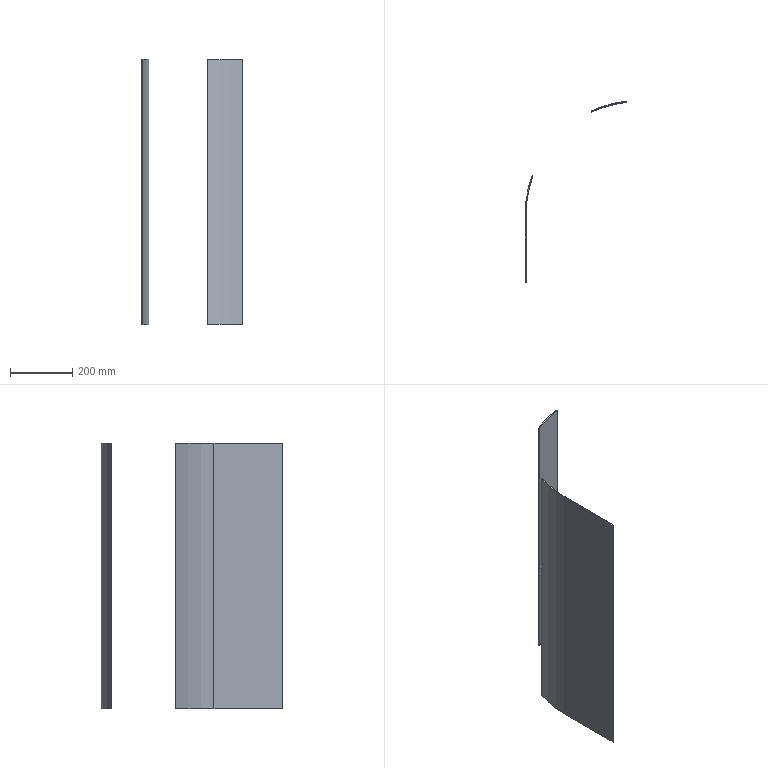Part | NX | features BREP 2 | 2 solids | 14 faces | box 325 x 580.972 x 850 mm | volume 1182499 mm3 | plane 10 | cylinder 4 | commonest cylinder face diameters 720 x2 726 x2
STEP:
#1=CARTESIAN_POINT('',(-150.365,327.094,819.));
#2=VERTEX_POINT('',#1);
#3=CARTESIAN_POINT('',(-38.,357.989,819.));
#4=VERTEX_POINT('',#3);
#5=CARTESIAN_POINT('',(0.,0.,819.));
#6=DIRECTION('',(0.,0.,-1.));
#7=DIRECTION('',(1.,0.,0.));
#8=AXIS2_PLACEMENT_3D('',#5,#6,#7);
#9=CIRCLE('',#8,360.);
#10=EDGE_CURVE('',#2,#4,#9,.T.);
#11=ORIENTED_EDGE('',*,*,#10,.F.);
#12=CARTESIAN_POINT('',(-150.365,327.094,-31.));
#13=VERTEX_POINT('',#12);
#14=CARTESIAN_POINT('',(-150.365,327.094,-31.));
#15=DIRECTION('',(0.,0.,1.));
#16=VECTOR('',#15,1000.);
#17=LINE('',#14,#16);
#18=EDGE_CURVE('',#13,#2,#17,.T.);
#19=ORIENTED_EDGE('',*,*,#18,.F.);
#20=CARTESIAN_POINT('',(-38.,357.989,-31.));
#21=VERTEX_POINT('',#20);
#22=CARTESIAN_POINT('',(0.,0.,-31.));
#23=DIRECTION('',(0.,0.,-1.));
#24=DIRECTION('',(1.,0.,0.));
#25=AXIS2_PLACEMENT_3D('',#22,#23,#24);
#26=CIRCLE('',#25,360.);
#27=EDGE_CURVE('',#13,#21,#26,.T.);
#28=ORIENTED_EDGE('',*,*,#27,.T.);
#29=CARTESIAN_POINT('',(-38.,357.989,819.));
#30=DIRECTION('',(0.,0.,-1.));
#31=VECTOR('',#30,1000.);
#32=LINE('',#29,#31);
#33=EDGE_CURVE('',#4,#21,#32,.T.);
#34=ORIENTED_EDGE('',*,*,#33,.F.);
#35=EDGE_LOOP('',(#11,#19,#28,#34));
#36=FACE_BOUND('',#35,.T.);
#37=CARTESIAN_POINT('',(0.,0.,819.));
#38=DIRECTION('',(0.,0.,-1.));
#39=DIRECTION('',(1.,0.,0.));
#40=AXIS2_PLACEMENT_3D('',#37,#38,#39);
#41=CYLINDRICAL_SURFACE('',#40,360.);
#42=ADVANCED_FACE('',(#36),#41,.F.);
#43=CARTESIAN_POINT('',(-151.618,329.82,-31.));
#44=VERTEX_POINT('',#43);
#45=CARTESIAN_POINT('',(-151.618,329.82,819.));
#46=VERTEX_POINT('',#45);
#47=CARTESIAN_POINT('',(-151.618,329.82,-31.));
#48=DIRECTION('',(0.,0.,1.));
#49=VECTOR('',#48,1000.);
#50=LINE('',#47,#49);
#51=EDGE_CURVE('',#44,#46,#50,.T.);
#52=ORIENTED_EDGE('',*,*,#51,.T.);
#53=CARTESIAN_POINT('',(-38.317,360.972,819.));
#54=VERTEX_POINT('',#53);
#55=CARTESIAN_POINT('',(0.,0.,819.));
#56=DIRECTION('',(0.,0.,-1.));
#57=DIRECTION('',(1.,0.,0.));
#58=AXIS2_PLACEMENT_3D('',#55,#56,#57);
#59=CIRCLE('',#58,363.);
#60=EDGE_CURVE('',#46,#54,#59,.T.);
#61=ORIENTED_EDGE('',*,*,#60,.T.);
#62=CARTESIAN_POINT('',(-38.317,360.972,-31.));
#63=VERTEX_POINT('',#62);
#64=CARTESIAN_POINT('',(-38.317,360.972,819.));
#65=DIRECTION('',(0.,0.,-1.));
#66=VECTOR('',#65,1000.);
#67=LINE('',#64,#66);
#68=EDGE_CURVE('',#54,#63,#67,.T.);
#69=ORIENTED_EDGE('',*,*,#68,.T.);
#70=CARTESIAN_POINT('',(0.,0.,-31.));
#71=DIRECTION('',(0.,0.,-1.));
#72=DIRECTION('',(1.,0.,0.));
#73=AXIS2_PLACEMENT_3D('',#70,#71,#72);
#74=CIRCLE('',#73,363.);
#75=EDGE_CURVE('',#44,#63,#74,.T.);
#76=ORIENTED_EDGE('',*,*,#75,.F.);
#77=EDGE_LOOP('',(#52,#61,#69,#76));
#78=FACE_BOUND('',#77,.T.);
#79=CARTESIAN_POINT('',(0.,0.,819.));
#80=DIRECTION('',(0.,0.,-1.));
#81=DIRECTION('',(1.,0.,0.));
#82=AXIS2_PLACEMENT_3D('',#79,#80,#81);
#83=CYLINDRICAL_SURFACE('',#82,363.);
#84=ADVANCED_FACE('',(#78),#83,.T.);
#85=ORIENTED_EDGE('',*,*,#60,.F.);
#86=CARTESIAN_POINT('',(-151.618,329.82,819.));
#87=DIRECTION('',(-0.4177,0.9086,0.));
#88=VECTOR('',#87,1000.);
#89=LINE('',#86,#88);
#90=EDGE_CURVE('',#2,#46,#89,.T.);
#91=ORIENTED_EDGE('',*,*,#90,.F.);
#92=ORIENTED_EDGE('',*,*,#10,.T.);
#93=CARTESIAN_POINT('',(-38.317,360.972,819.));
#94=DIRECTION('',(0.1056,-0.9944,0.));
#95=VECTOR('',#94,1000.);
#96=LINE('',#93,#95);
#97=EDGE_CURVE('',#54,#4,#96,.T.);
#98=ORIENTED_EDGE('',*,*,#97,.F.);
#99=EDGE_LOOP('',(#85,#91,#92,#98));
#100=FACE_BOUND('',#99,.T.);
#101=CARTESIAN_POINT('',(0.,0.,819.));
#102=DIRECTION('',(0.,0.,-1.));
#103=DIRECTION('',(1.,0.,0.));
#104=AXIS2_PLACEMENT_3D('',#101,#102,#103);
#105=PLANE('',#104);
#106=ADVANCED_FACE('',(#100),#105,.F.);
#107=CARTESIAN_POINT('',(-151.618,329.82,-31.));
#108=DIRECTION('',(-0.4177,0.9086,0.));
#109=VECTOR('',#108,1000.);
#110=LINE('',#107,#109);
#111=EDGE_CURVE('',#13,#44,#110,.T.);
#112=ORIENTED_EDGE('',*,*,#111,.T.);
#113=ORIENTED_EDGE('',*,*,#75,.T.);
#114=CARTESIAN_POINT('',(-38.317,360.972,-31.));
#115=DIRECTION('',(0.1056,-0.9944,0.));
#116=VECTOR('',#115,1000.);
#117=LINE('',#114,#116);
#118=EDGE_CURVE('',#63,#21,#117,.T.);
#119=ORIENTED_EDGE('',*,*,#118,.T.);
#120=ORIENTED_EDGE('',*,*,#27,.F.);
#121=EDGE_LOOP('',(#112,#113,#119,#120));
#122=FACE_BOUND('',#121,.T.);
#123=CARTESIAN_POINT('',(0.,0.,-31.));
#124=DIRECTION('',(0.,0.,-1.));
#125=DIRECTION('',(1.,0.,0.));
#126=AXIS2_PLACEMENT_3D('',#123,#124,#125);
#127=PLANE('',#126);
#128=ADVANCED_FACE('',(#122),#127,.T.);
#129=ORIENTED_EDGE('',*,*,#118,.F.);
#130=ORIENTED_EDGE('',*,*,#68,.F.);
#131=ORIENTED_EDGE('',*,*,#97,.T.);
#132=ORIENTED_EDGE('',*,*,#33,.T.);
#133=EDGE_LOOP('',(#129,#130,#131,#132));
#134=FACE_BOUND('',#133,.T.);
#135=CARTESIAN_POINT('',(-38.317,360.972,819.));
#136=DIRECTION('',(0.9944,0.1056,0.));
#137=DIRECTION('',(0.1056,-0.9944,0.));
#138=AXIS2_PLACEMENT_3D('',#135,#136,#137);
#139=PLANE('',#138);
#140=ADVANCED_FACE('',(#134),#139,.T.);
#141=ORIENTED_EDGE('',*,*,#90,.T.);
#142=ORIENTED_EDGE('',*,*,#51,.F.);
#143=ORIENTED_EDGE('',*,*,#111,.F.);
#144=ORIENTED_EDGE('',*,*,#18,.T.);
#145=EDGE_LOOP('',(#141,#142,#143,#144));
#146=FACE_BOUND('',#145,.T.);
#147=CARTESIAN_POINT('',(-151.618,329.82,-31.));
#148=DIRECTION('',(0.9086,0.4177,0.));
#149=DIRECTION('',(0.4177,-0.9086,0.));
#150=AXIS2_PLACEMENT_3D('',#147,#148,#149);
#151=PLANE('',#150);
#152=ADVANCED_FACE('',(#146),#151,.F.);
#153=CLOSED_SHELL('',(#42,#84,#106,#128,#140,#152));
#154=MANIFOLD_SOLID_BREP('',#153);
#155=CARTESIAN_POINT('',(-363.,-220.,-31.));
#156=VERTEX_POINT('',#155);
#157=CARTESIAN_POINT('',(-363.,0.,-31.));
#158=VERTEX_POINT('',#157);
#159=CARTESIAN_POINT('',(-363.,-220.,-31.));
#160=DIRECTION('',(0.,1.,0.));
#161=VECTOR('',#160,1000.);
#162=LINE('',#159,#161);
#163=EDGE_CURVE('',#156,#158,#162,.T.);
#164=ORIENTED_EDGE('',*,*,#163,.F.);
#165=CARTESIAN_POINT('',(-363.,-220.,819.));
#166=VERTEX_POINT('',#165);
#167=CARTESIAN_POINT('',(-363.,-220.,819.));
#168=DIRECTION('',(0.,0.,-1.));
#169=VECTOR('',#168,1000.);
#170=LINE('',#167,#169);
#171=EDGE_CURVE('',#166,#156,#170,.T.);
#172=ORIENTED_EDGE('',*,*,#171,.F.);
#173=CARTESIAN_POINT('',(-363.,0.,819.));
#174=VERTEX_POINT('',#173);
#175=CARTESIAN_POINT('',(-363.,-220.,819.));
#176=DIRECTION('',(0.,1.,0.));
#177=VECTOR('',#176,1000.);
#178=LINE('',#175,#177);
#179=EDGE_CURVE('',#166,#174,#178,.T.);
#180=ORIENTED_EDGE('',*,*,#179,.T.);
#181=CARTESIAN_POINT('',(-363.,0.,819.));
#182=DIRECTION('',(0.,0.,-1.));
#183=VECTOR('',#182,1000.);
#184=LINE('',#181,#183);
#185=EDGE_CURVE('',#174,#158,#184,.T.);
#186=ORIENTED_EDGE('',*,*,#185,.T.);
#187=EDGE_LOOP('',(#164,#172,#180,#186));
#188=FACE_BOUND('',#187,.T.);
#189=CARTESIAN_POINT('',(-363.,-220.,819.));
#190=DIRECTION('',(-1.,0.,0.));
#191=DIRECTION('',(0.,0.,-1.));
#192=AXIS2_PLACEMENT_3D('',#189,#190,#191);
#193=PLANE('',#192);
#194=ADVANCED_FACE('',(#188),#193,.T.);
#195=CARTESIAN_POINT('',(-360.,-220.,-31.));
#196=VERTEX_POINT('',#195);
#197=CARTESIAN_POINT('',(-360.,-220.,-31.));
#198=DIRECTION('',(-1.,0.,0.));
#199=VECTOR('',#198,1000.);
#200=LINE('',#197,#199);
#201=EDGE_CURVE('',#196,#156,#200,.T.);
#202=ORIENTED_EDGE('',*,*,#201,.F.);
#203=CARTESIAN_POINT('',(-360.,-220.,819.));
#204=VERTEX_POINT('',#203);
#205=CARTESIAN_POINT('',(-360.,-220.,819.));
#206=DIRECTION('',(0.,0.,-1.));
#207=VECTOR('',#206,1000.);
#208=LINE('',#205,#207);
#209=EDGE_CURVE('',#204,#196,#208,.T.);
#210=ORIENTED_EDGE('',*,*,#209,.F.);
#211=CARTESIAN_POINT('',(-360.,-220.,819.));
#212=DIRECTION('',(-1.,0.,0.));
#213=VECTOR('',#212,1000.);
#214=LINE('',#211,#213);
#215=EDGE_CURVE('',#204,#166,#214,.T.);
#216=ORIENTED_EDGE('',*,*,#215,.T.);
#217=ORIENTED_EDGE('',*,*,#171,.T.);
#218=EDGE_LOOP('',(#202,#210,#216,#217));
#219=FACE_BOUND('',#218,.T.);
#220=CARTESIAN_POINT('',(-360.,-220.,819.));
#221=DIRECTION('',(0.,-1.,0.));
#222=DIRECTION('',(0.,0.,1.));
#223=AXIS2_PLACEMENT_3D('',#220,#221,#222);
#224=PLANE('',#223);
#225=ADVANCED_FACE('',(#219),#224,.T.);
#226=CARTESIAN_POINT('',(-360.,0.,-31.));
#227=VERTEX_POINT('',#226);
#228=CARTESIAN_POINT('',(-360.,-220.,-31.));
#229=DIRECTION('',(0.,1.,0.));
#230=VECTOR('',#229,1000.);
#231=LINE('',#228,#230);
#232=EDGE_CURVE('',#196,#227,#231,.T.);
#233=ORIENTED_EDGE('',*,*,#232,.T.);
#234=CARTESIAN_POINT('',(-360.,0.,819.));
#235=VERTEX_POINT('',#234);
#236=CARTESIAN_POINT('',(-360.,0.,819.));
#237=DIRECTION('',(0.,0.,-1.));
#238=VECTOR('',#237,1000.);
#239=LINE('',#236,#238);
#240=EDGE_CURVE('',#235,#227,#239,.T.);
#241=ORIENTED_EDGE('',*,*,#240,.F.);
#242=CARTESIAN_POINT('',(-360.,-220.,819.));
#243=DIRECTION('',(0.,1.,0.));
#244=VECTOR('',#243,1000.);
#245=LINE('',#242,#244);
#246=EDGE_CURVE('',#204,#235,#245,.T.);
#247=ORIENTED_EDGE('',*,*,#246,.F.);
#248=ORIENTED_EDGE('',*,*,#209,.T.);
#249=EDGE_LOOP('',(#233,#241,#247,#248));
#250=FACE_BOUND('',#249,.T.);
#251=CARTESIAN_POINT('',(-360.,-220.,819.));
#252=DIRECTION('',(-1.,0.,0.));
#253=DIRECTION('',(0.,0.,-1.));
#254=AXIS2_PLACEMENT_3D('',#251,#252,#253);
#255=PLANE('',#254);
#256=ADVANCED_FACE('',(#250),#255,.F.);
#257=CARTESIAN_POINT('',(-338.289,123.127,819.));
#258=VERTEX_POINT('',#257);
#259=CARTESIAN_POINT('',(0.,0.,819.));
#260=DIRECTION('',(0.,0.,-1.));
#261=DIRECTION('',(1.,0.,0.));
#262=AXIS2_PLACEMENT_3D('',#259,#260,#261);
#263=CIRCLE('',#262,360.);
#264=EDGE_CURVE('',#235,#258,#263,.T.);
#265=ORIENTED_EDGE('',*,*,#264,.T.);
#266=CARTESIAN_POINT('',(-341.108,124.153,819.));
#267=VERTEX_POINT('',#266);
#268=CARTESIAN_POINT('',(-341.108,124.153,819.));
#269=DIRECTION('',(0.9397,-0.342,0.));
#270=VECTOR('',#269,1000.);
#271=LINE('',#268,#270);
#272=EDGE_CURVE('',#267,#258,#271,.T.);
#273=ORIENTED_EDGE('',*,*,#272,.F.);
#274=CARTESIAN_POINT('',(0.,0.,819.));
#275=DIRECTION('',(0.,0.,-1.));
#276=DIRECTION('',(1.,0.,0.));
#277=AXIS2_PLACEMENT_3D('',#274,#275,#276);
#278=CIRCLE('',#277,363.);
#279=EDGE_CURVE('',#174,#267,#278,.T.);
#280=ORIENTED_EDGE('',*,*,#279,.F.);
#281=ORIENTED_EDGE('',*,*,#179,.F.);
#282=ORIENTED_EDGE('',*,*,#215,.F.);
#283=ORIENTED_EDGE('',*,*,#246,.T.);
#284=EDGE_LOOP('',(#265,#273,#280,#281,#282,#283));
#285=FACE_BOUND('',#284,.T.);
#286=CARTESIAN_POINT('',(0.,0.,819.));
#287=DIRECTION('',(0.,0.,-1.));
#288=DIRECTION('',(1.,0.,0.));
#289=AXIS2_PLACEMENT_3D('',#286,#287,#288);
#290=PLANE('',#289);
#291=ADVANCED_FACE('',(#285),#290,.F.);
#292=CARTESIAN_POINT('',(-341.108,124.153,-31.));
#293=VERTEX_POINT('',#292);
#294=CARTESIAN_POINT('',(-338.289,123.127,-31.));
#295=VERTEX_POINT('',#294);
#296=CARTESIAN_POINT('',(-341.108,124.153,-31.));
#297=DIRECTION('',(0.9397,-0.342,0.));
#298=VECTOR('',#297,1000.);
#299=LINE('',#296,#298);
#300=EDGE_CURVE('',#293,#295,#299,.T.);
#301=ORIENTED_EDGE('',*,*,#300,.T.);
#302=CARTESIAN_POINT('',(0.,0.,-31.));
#303=DIRECTION('',(0.,0.,-1.));
#304=DIRECTION('',(1.,0.,0.));
#305=AXIS2_PLACEMENT_3D('',#302,#303,#304);
#306=CIRCLE('',#305,360.);
#307=EDGE_CURVE('',#227,#295,#306,.T.);
#308=ORIENTED_EDGE('',*,*,#307,.F.);
#309=ORIENTED_EDGE('',*,*,#232,.F.);
#310=ORIENTED_EDGE('',*,*,#201,.T.);
#311=ORIENTED_EDGE('',*,*,#163,.T.);
#312=CARTESIAN_POINT('',(0.,0.,-31.));
#313=DIRECTION('',(0.,0.,-1.));
#314=DIRECTION('',(1.,0.,0.));
#315=AXIS2_PLACEMENT_3D('',#312,#313,#314);
#316=CIRCLE('',#315,363.);
#317=EDGE_CURVE('',#158,#293,#316,.T.);
#318=ORIENTED_EDGE('',*,*,#317,.T.);
#319=EDGE_LOOP('',(#301,#308,#309,#310,#311,#318));
#320=FACE_BOUND('',#319,.T.);
#321=CARTESIAN_POINT('',(0.,0.,-31.));
#322=DIRECTION('',(0.,0.,-1.));
#323=DIRECTION('',(1.,0.,0.));
#324=AXIS2_PLACEMENT_3D('',#321,#322,#323);
#325=PLANE('',#324);
#326=ADVANCED_FACE('',(#320),#325,.T.);
#327=CARTESIAN_POINT('',(-341.108,124.153,-31.));
#328=DIRECTION('',(0.,0.,1.));
#329=VECTOR('',#328,1000.);
#330=LINE('',#327,#329);
#331=EDGE_CURVE('',#293,#267,#330,.T.);
#332=ORIENTED_EDGE('',*,*,#331,.F.);
#333=ORIENTED_EDGE('',*,*,#317,.F.);
#334=ORIENTED_EDGE('',*,*,#185,.F.);
#335=ORIENTED_EDGE('',*,*,#279,.T.);
#336=EDGE_LOOP('',(#332,#333,#334,#335));
#337=FACE_BOUND('',#336,.T.);
#338=CARTESIAN_POINT('',(0.,0.,819.));
#339=DIRECTION('',(0.,0.,-1.));
#340=DIRECTION('',(1.,0.,0.));
#341=AXIS2_PLACEMENT_3D('',#338,#339,#340);
#342=CYLINDRICAL_SURFACE('',#341,363.);
#343=ADVANCED_FACE('',(#337),#342,.T.);
#344=ORIENTED_EDGE('',*,*,#307,.T.);
#345=CARTESIAN_POINT('',(-338.289,123.127,-31.));
#346=DIRECTION('',(0.,0.,1.));
#347=VECTOR('',#346,1000.);
#348=LINE('',#345,#347);
#349=EDGE_CURVE('',#295,#258,#348,.T.);
#350=ORIENTED_EDGE('',*,*,#349,.T.);
#351=ORIENTED_EDGE('',*,*,#264,.F.);
#352=ORIENTED_EDGE('',*,*,#240,.T.);
#353=EDGE_LOOP('',(#344,#350,#351,#352));
#354=FACE_BOUND('',#353,.T.);
#355=CARTESIAN_POINT('',(0.,0.,819.));
#356=DIRECTION('',(0.,0.,-1.));
#357=DIRECTION('',(1.,0.,0.));
#358=AXIS2_PLACEMENT_3D('',#355,#356,#357);
#359=CYLINDRICAL_SURFACE('',#358,360.);
#360=ADVANCED_FACE('',(#354),#359,.F.);
#361=ORIENTED_EDGE('',*,*,#272,.T.);
#362=ORIENTED_EDGE('',*,*,#349,.F.);
#363=ORIENTED_EDGE('',*,*,#300,.F.);
#364=ORIENTED_EDGE('',*,*,#331,.T.);
#365=EDGE_LOOP('',(#361,#362,#363,#364));
#366=FACE_BOUND('',#365,.T.);
#367=CARTESIAN_POINT('',(-341.108,124.153,-31.));
#368=DIRECTION('',(-0.342,-0.9397,0.));
#369=DIRECTION('',(-0.9397,0.342,0.));
#370=AXIS2_PLACEMENT_3D('',#367,#368,#369);
#371=PLANE('',#370);
#372=ADVANCED_FACE('',(#366),#371,.F.);
#373=CLOSED_SHELL('',(#194,#225,#256,#291,#326,#343,#360,#372));
#374=MANIFOLD_SOLID_BREP('',#373);
#375=(LENGTH_UNIT()NAMED_UNIT(*)SI_UNIT(.MILLI.,.METRE.));
#376=UNCERTAINTY_MEASURE_WITH_UNIT(LENGTH_MEASURE(0.00001),#375,'','');
#377=(NAMED_UNIT(*)PLANE_ANGLE_UNIT()SI_UNIT($,.RADIAN.));
#378=(NAMED_UNIT(*)SI_UNIT($,.STERADIAN.)SOLID_ANGLE_UNIT());
#379=(GEOMETRIC_REPRESENTATION_CONTEXT(3)GLOBAL_UNCERTAINTY_ASSIGNED_CONTEXT((#376))GLOBAL_UNIT_ASSIGNED_CONTEXT((#375,#377,#378))REPRESENTATION_CONTEXT('',''));
#380=ADVANCED_BREP_SHAPE_REPRESENTATION('',(#154,#374),#379);